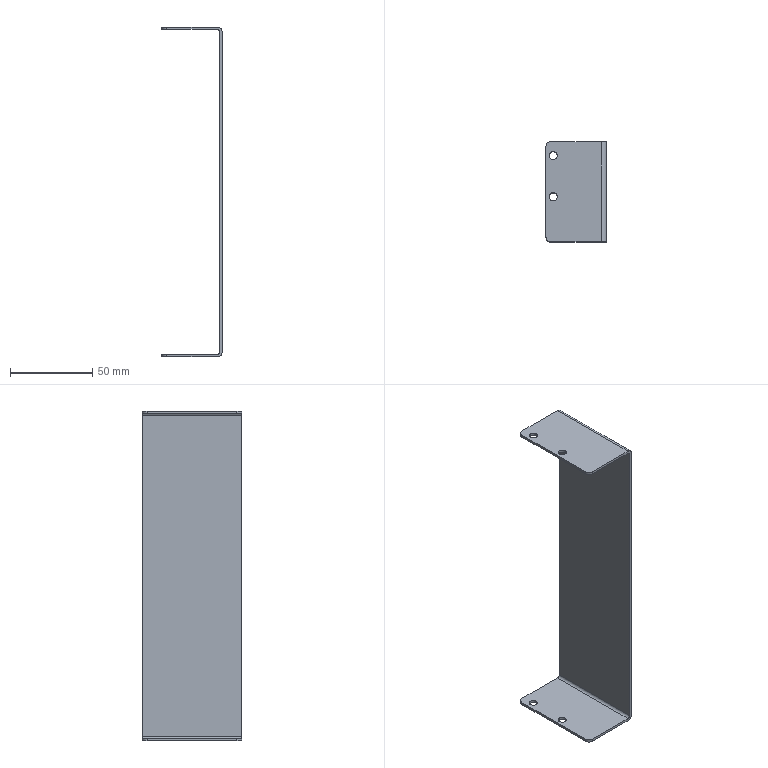Part | SolidWorks | features BaseBody 1 | 1 solid | 26 faces | box 36.5 x 60.5 x 200 mm | volume 24198 mm3 | cylinder 16 | plane 10 | commonest cylinder face diameters 5 x8 6 x6 3 x2
STEP:
#1=CARTESIAN_POINT('',(310.979,1928.044,-20.5));
#2=VERTEX_POINT('',#1);
#3=CARTESIAN_POINT('',(305.979,1928.044,-20.5));
#4=VERTEX_POINT('',#3);
#5=CARTESIAN_POINT('',(308.479,1928.044,-20.5));
#6=DIRECTION('',(0.,0.,-1.));
#7=DIRECTION('',(-1.,0.,0.));
#8=AXIS2_PLACEMENT_3D('',#5,#6,#7);
#9=CIRCLE('',#8,2.5);
#10=EDGE_CURVE('',#2,#4,#9,.T.);
#11=ORIENTED_EDGE('',*,*,#10,.F.);
#12=CARTESIAN_POINT('',(310.979,1928.044,-22.));
#13=VERTEX_POINT('',#12);
#14=CARTESIAN_POINT('',(310.979,1928.044,-8.386));
#15=DIRECTION('',(0.,0.,-1.));
#16=VECTOR('',#15,1000.);
#17=LINE('',#14,#16);
#18=EDGE_CURVE('',#2,#13,#17,.T.);
#19=ORIENTED_EDGE('',*,*,#18,.T.);
#20=CARTESIAN_POINT('',(305.979,1928.044,-22.));
#21=VERTEX_POINT('',#20);
#22=CARTESIAN_POINT('',(308.479,1928.044,-22.));
#23=DIRECTION('',(0.,0.,-1.));
#24=DIRECTION('',(-1.,0.,0.));
#25=AXIS2_PLACEMENT_3D('',#22,#23,#24);
#26=CIRCLE('',#25,2.5);
#27=EDGE_CURVE('',#13,#21,#26,.T.);
#28=ORIENTED_EDGE('',*,*,#27,.T.);
#29=CARTESIAN_POINT('',(305.979,1928.044,-8.386));
#30=DIRECTION('',(0.,0.,-1.));
#31=VECTOR('',#30,1000.);
#32=LINE('',#29,#31);
#33=EDGE_CURVE('',#4,#21,#32,.T.);
#34=ORIENTED_EDGE('',*,*,#33,.F.);
#35=EDGE_LOOP('',(#11,#19,#28,#34));
#36=FACE_OUTER_BOUND('',#35,.T.);
#37=CARTESIAN_POINT('',(308.479,1928.044,-8.386));
#38=DIRECTION('',(0.,0.,-1.));
#39=DIRECTION('',(-1.,0.,0.));
#40=AXIS2_PLACEMENT_3D('',#37,#38,#39);
#41=CYLINDRICAL_SURFACE('',#40,2.5);
#42=ADVANCED_FACE('',(#36),#41,.F.);
#43=CARTESIAN_POINT('',(310.979,1903.044,-20.5));
#44=VERTEX_POINT('',#43);
#45=CARTESIAN_POINT('',(305.979,1903.044,-20.5));
#46=VERTEX_POINT('',#45);
#47=CARTESIAN_POINT('',(308.479,1903.044,-20.5));
#48=DIRECTION('',(0.,0.,-1.));
#49=DIRECTION('',(-1.,0.,0.));
#50=AXIS2_PLACEMENT_3D('',#47,#48,#49);
#51=CIRCLE('',#50,2.5);
#52=EDGE_CURVE('',#44,#46,#51,.T.);
#53=ORIENTED_EDGE('',*,*,#52,.F.);
#54=CARTESIAN_POINT('',(310.979,1903.044,-22.));
#55=VERTEX_POINT('',#54);
#56=CARTESIAN_POINT('',(310.979,1903.044,-8.386));
#57=DIRECTION('',(0.,0.,-1.));
#58=VECTOR('',#57,1000.);
#59=LINE('',#56,#58);
#60=EDGE_CURVE('',#44,#55,#59,.T.);
#61=ORIENTED_EDGE('',*,*,#60,.T.);
#62=CARTESIAN_POINT('',(305.979,1903.044,-22.));
#63=VERTEX_POINT('',#62);
#64=CARTESIAN_POINT('',(308.479,1903.044,-22.));
#65=DIRECTION('',(0.,0.,-1.));
#66=DIRECTION('',(-1.,0.,0.));
#67=AXIS2_PLACEMENT_3D('',#64,#65,#66);
#68=CIRCLE('',#67,2.5);
#69=EDGE_CURVE('',#55,#63,#68,.T.);
#70=ORIENTED_EDGE('',*,*,#69,.T.);
#71=CARTESIAN_POINT('',(305.979,1903.044,-8.386));
#72=DIRECTION('',(0.,0.,-1.));
#73=VECTOR('',#72,1000.);
#74=LINE('',#71,#73);
#75=EDGE_CURVE('',#46,#63,#74,.T.);
#76=ORIENTED_EDGE('',*,*,#75,.F.);
#77=EDGE_LOOP('',(#53,#61,#70,#76));
#78=FACE_OUTER_BOUND('',#77,.T.);
#79=CARTESIAN_POINT('',(308.479,1903.044,-8.386));
#80=DIRECTION('',(0.,0.,-1.));
#81=DIRECTION('',(-1.,0.,0.));
#82=AXIS2_PLACEMENT_3D('',#79,#80,#81);
#83=CYLINDRICAL_SURFACE('',#82,2.5);
#84=ADVANCED_FACE('',(#78),#83,.F.);
#85=CARTESIAN_POINT('',(310.979,1928.044,-219.));
#86=VERTEX_POINT('',#85);
#87=CARTESIAN_POINT('',(305.979,1928.044,-219.));
#88=VERTEX_POINT('',#87);
#89=CARTESIAN_POINT('',(308.479,1928.044,-219.));
#90=DIRECTION('',(0.,0.,-1.));
#91=DIRECTION('',(-1.,0.,0.));
#92=AXIS2_PLACEMENT_3D('',#89,#90,#91);
#93=CIRCLE('',#92,2.5);
#94=EDGE_CURVE('',#86,#88,#93,.T.);
#95=ORIENTED_EDGE('',*,*,#94,.F.);
#96=CARTESIAN_POINT('',(310.979,1928.044,-220.5));
#97=VERTEX_POINT('',#96);
#98=CARTESIAN_POINT('',(310.979,1928.044,-8.386));
#99=DIRECTION('',(0.,0.,-1.));
#100=VECTOR('',#99,1000.);
#101=LINE('',#98,#100);
#102=EDGE_CURVE('',#86,#97,#101,.T.);
#103=ORIENTED_EDGE('',*,*,#102,.T.);
#104=CARTESIAN_POINT('',(305.979,1928.044,-220.5));
#105=VERTEX_POINT('',#104);
#106=CARTESIAN_POINT('',(308.479,1928.044,-220.5));
#107=DIRECTION('',(0.,0.,-1.));
#108=DIRECTION('',(-1.,0.,0.));
#109=AXIS2_PLACEMENT_3D('',#106,#107,#108);
#110=CIRCLE('',#109,2.5);
#111=EDGE_CURVE('',#97,#105,#110,.T.);
#112=ORIENTED_EDGE('',*,*,#111,.T.);
#113=CARTESIAN_POINT('',(305.979,1928.044,-8.386));
#114=DIRECTION('',(0.,0.,-1.));
#115=VECTOR('',#114,1000.);
#116=LINE('',#113,#115);
#117=EDGE_CURVE('',#88,#105,#116,.T.);
#118=ORIENTED_EDGE('',*,*,#117,.F.);
#119=EDGE_LOOP('',(#95,#103,#112,#118));
#120=FACE_OUTER_BOUND('',#119,.T.);
#121=CARTESIAN_POINT('',(308.479,1928.044,-8.386));
#122=DIRECTION('',(0.,0.,-1.));
#123=DIRECTION('',(-1.,0.,0.));
#124=AXIS2_PLACEMENT_3D('',#121,#122,#123);
#125=CYLINDRICAL_SURFACE('',#124,2.5);
#126=ADVANCED_FACE('',(#120),#125,.F.);
#127=CARTESIAN_POINT('',(310.979,1903.044,-219.));
#128=VERTEX_POINT('',#127);
#129=CARTESIAN_POINT('',(305.979,1903.044,-219.));
#130=VERTEX_POINT('',#129);
#131=CARTESIAN_POINT('',(308.479,1903.044,-219.));
#132=DIRECTION('',(0.,0.,-1.));
#133=DIRECTION('',(-1.,0.,0.));
#134=AXIS2_PLACEMENT_3D('',#131,#132,#133);
#135=CIRCLE('',#134,2.5);
#136=EDGE_CURVE('',#128,#130,#135,.T.);
#137=ORIENTED_EDGE('',*,*,#136,.F.);
#138=CARTESIAN_POINT('',(310.979,1903.044,-220.5));
#139=VERTEX_POINT('',#138);
#140=CARTESIAN_POINT('',(310.979,1903.044,-8.386));
#141=DIRECTION('',(0.,0.,-1.));
#142=VECTOR('',#141,1000.);
#143=LINE('',#140,#142);
#144=EDGE_CURVE('',#128,#139,#143,.T.);
#145=ORIENTED_EDGE('',*,*,#144,.T.);
#146=CARTESIAN_POINT('',(305.979,1903.044,-220.5));
#147=VERTEX_POINT('',#146);
#148=CARTESIAN_POINT('',(308.479,1903.044,-220.5));
#149=DIRECTION('',(0.,0.,-1.));
#150=DIRECTION('',(-1.,0.,0.));
#151=AXIS2_PLACEMENT_3D('',#148,#149,#150);
#152=CIRCLE('',#151,2.5);
#153=EDGE_CURVE('',#139,#147,#152,.T.);
#154=ORIENTED_EDGE('',*,*,#153,.T.);
#155=CARTESIAN_POINT('',(305.979,1903.044,-8.386));
#156=DIRECTION('',(0.,0.,-1.));
#157=VECTOR('',#156,1000.);
#158=LINE('',#155,#157);
#159=EDGE_CURVE('',#130,#147,#158,.T.);
#160=ORIENTED_EDGE('',*,*,#159,.F.);
#161=EDGE_LOOP('',(#137,#145,#154,#160));
#162=FACE_OUTER_BOUND('',#161,.T.);
#163=CARTESIAN_POINT('',(308.479,1903.044,-8.386));
#164=DIRECTION('',(0.,0.,-1.));
#165=DIRECTION('',(-1.,0.,0.));
#166=AXIS2_PLACEMENT_3D('',#163,#164,#165);
#167=CYLINDRICAL_SURFACE('',#166,2.5);
#168=ADVANCED_FACE('',(#162),#167,.F.);
#169=CARTESIAN_POINT('',(340.479,1936.294,-217.5));
#170=VERTEX_POINT('',#169);
#171=CARTESIAN_POINT('',(340.479,1936.294,-23.5));
#172=VERTEX_POINT('',#171);
#173=CARTESIAN_POINT('',(340.479,1936.294,-120.5));
#174=DIRECTION('',(0.,0.,1.));
#175=VECTOR('',#174,1000.);
#176=LINE('',#173,#175);
#177=EDGE_CURVE('',#170,#172,#176,.T.);
#178=ORIENTED_EDGE('',*,*,#177,.T.);
#179=CARTESIAN_POINT('',(340.479,1875.794,-23.5));
#180=VERTEX_POINT('',#179);
#181=CARTESIAN_POINT('',(340.479,1906.044,-23.5));
#182=DIRECTION('',(0.,-1.,0.));
#183=VECTOR('',#182,1000.);
#184=LINE('',#181,#183);
#185=EDGE_CURVE('',#172,#180,#184,.T.);
#186=ORIENTED_EDGE('',*,*,#185,.T.);
#187=CARTESIAN_POINT('',(340.479,1875.794,-217.5));
#188=VERTEX_POINT('',#187);
#189=CARTESIAN_POINT('',(340.479,1875.794,-120.5));
#190=DIRECTION('',(0.,0.,-1.));
#191=VECTOR('',#190,1000.);
#192=LINE('',#189,#191);
#193=EDGE_CURVE('',#180,#188,#192,.T.);
#194=ORIENTED_EDGE('',*,*,#193,.T.);
#195=CARTESIAN_POINT('',(340.479,1906.044,-217.5));
#196=DIRECTION('',(0.,1.,0.));
#197=VECTOR('',#196,1000.);
#198=LINE('',#195,#197);
#199=EDGE_CURVE('',#188,#170,#198,.T.);
#200=ORIENTED_EDGE('',*,*,#199,.T.);
#201=EDGE_LOOP('',(#178,#186,#194,#200));
#202=FACE_OUTER_BOUND('',#201,.T.);
#203=CARTESIAN_POINT('',(340.479,1906.044,-120.5));
#204=DIRECTION('',(1.,0.,0.));
#205=DIRECTION('',(0.,0.,-1.));
#206=AXIS2_PLACEMENT_3D('',#203,#204,#205);
#207=PLANE('',#206);
#208=ADVANCED_FACE('',(#202),#207,.T.);
#209=CARTESIAN_POINT('',(337.479,1875.794,-20.5));
#210=VERTEX_POINT('',#209);
#211=CARTESIAN_POINT('',(337.479,1875.794,-23.5));
#212=DIRECTION('',(0.,1.,0.));
#213=DIRECTION('',(0.,0.,-1.));
#214=AXIS2_PLACEMENT_3D('',#211,#212,#213);
#215=CIRCLE('',#214,3.);
#216=EDGE_CURVE('',#210,#180,#215,.T.);
#217=ORIENTED_EDGE('',*,*,#216,.T.);
#218=ORIENTED_EDGE('',*,*,#185,.F.);
#219=CARTESIAN_POINT('',(337.479,1936.294,-20.5));
#220=VERTEX_POINT('',#219);
#221=CARTESIAN_POINT('',(337.479,1936.294,-23.5));
#222=DIRECTION('',(0.,-1.,0.));
#223=DIRECTION('',(0.,0.,-1.));
#224=AXIS2_PLACEMENT_3D('',#221,#222,#223);
#225=CIRCLE('',#224,3.);
#226=EDGE_CURVE('',#172,#220,#225,.T.);
#227=ORIENTED_EDGE('',*,*,#226,.T.);
#228=CARTESIAN_POINT('',(337.479,1906.044,-20.5));
#229=DIRECTION('',(0.,-1.,0.));
#230=VECTOR('',#229,1000.);
#231=LINE('',#228,#230);
#232=EDGE_CURVE('',#220,#210,#231,.T.);
#233=ORIENTED_EDGE('',*,*,#232,.T.);
#234=EDGE_LOOP('',(#217,#218,#227,#233));
#235=FACE_OUTER_BOUND('',#234,.T.);
#236=CARTESIAN_POINT('',(337.479,1906.044,-23.5));
#237=DIRECTION('',(0.,-1.,0.));
#238=DIRECTION('',(0.,0.,-1.));
#239=AXIS2_PLACEMENT_3D('',#236,#237,#238);
#240=CYLINDRICAL_SURFACE('',#239,3.);
#241=ADVANCED_FACE('',(#235),#240,.T.);
#242=CARTESIAN_POINT('',(338.979,1936.294,-217.5));
#243=VERTEX_POINT('',#242);
#244=CARTESIAN_POINT('',(338.979,1936.294,-23.5));
#245=VERTEX_POINT('',#244);
#246=CARTESIAN_POINT('',(338.979,1936.294,-20.5));
#247=DIRECTION('',(0.,0.,1.));
#248=VECTOR('',#247,1000.);
#249=LINE('',#246,#248);
#250=EDGE_CURVE('',#243,#245,#249,.T.);
#251=ORIENTED_EDGE('',*,*,#250,.T.);
#252=CARTESIAN_POINT('',(337.479,1936.294,-22.));
#253=VERTEX_POINT('',#252);
#254=CARTESIAN_POINT('',(337.479,1936.294,-23.5));
#255=DIRECTION('',(0.,-1.,0.));
#256=DIRECTION('',(0.,0.,-1.));
#257=AXIS2_PLACEMENT_3D('',#254,#255,#256);
#258=CIRCLE('',#257,1.5);
#259=EDGE_CURVE('',#245,#253,#258,.T.);
#260=ORIENTED_EDGE('',*,*,#259,.T.);
#261=CARTESIAN_POINT('',(306.979,1936.294,-22.));
#262=VERTEX_POINT('',#261);
#263=CARTESIAN_POINT('',(338.979,1936.294,-22.));
#264=DIRECTION('',(-1.,0.,0.));
#265=VECTOR('',#264,1000.);
#266=LINE('',#263,#265);
#267=EDGE_CURVE('',#253,#262,#266,.T.);
#268=ORIENTED_EDGE('',*,*,#267,.T.);
#269=CARTESIAN_POINT('',(306.979,1936.294,-20.5));
#270=VERTEX_POINT('',#269);
#271=CARTESIAN_POINT('',(306.979,1936.294,-20.5));
#272=DIRECTION('',(0.,0.,1.));
#273=VECTOR('',#272,1000.);
#274=LINE('',#271,#273);
#275=EDGE_CURVE('',#262,#270,#274,.T.);
#276=ORIENTED_EDGE('',*,*,#275,.T.);
#277=CARTESIAN_POINT('',(338.979,1936.294,-20.5));
#278=DIRECTION('',(1.,0.,0.));
#279=VECTOR('',#278,1000.);
#280=LINE('',#277,#279);
#281=EDGE_CURVE('',#270,#220,#280,.T.);
#282=ORIENTED_EDGE('',*,*,#281,.T.);
#283=ORIENTED_EDGE('',*,*,#226,.F.);
#284=ORIENTED_EDGE('',*,*,#177,.F.);
#285=CARTESIAN_POINT('',(337.479,1936.294,-220.5));
#286=VERTEX_POINT('',#285);
#287=CARTESIAN_POINT('',(337.479,1936.294,-217.5));
#288=DIRECTION('',(0.,1.,0.));
#289=DIRECTION('',(0.,0.,1.));
#290=AXIS2_PLACEMENT_3D('',#287,#288,#289);
#291=CIRCLE('',#290,3.);
#292=EDGE_CURVE('',#170,#286,#291,.T.);
#293=ORIENTED_EDGE('',*,*,#292,.T.);
#294=CARTESIAN_POINT('',(306.979,1936.294,-220.5));
#295=VERTEX_POINT('',#294);
#296=CARTESIAN_POINT('',(338.979,1936.294,-220.5));
#297=DIRECTION('',(-1.,0.,0.));
#298=VECTOR('',#297,1000.);
#299=LINE('',#296,#298);
#300=EDGE_CURVE('',#286,#295,#299,.T.);
#301=ORIENTED_EDGE('',*,*,#300,.T.);
#302=CARTESIAN_POINT('',(306.979,1936.294,-219.));
#303=VERTEX_POINT('',#302);
#304=CARTESIAN_POINT('',(306.979,1936.294,-20.5));
#305=DIRECTION('',(0.,0.,1.));
#306=VECTOR('',#305,1000.);
#307=LINE('',#304,#306);
#308=EDGE_CURVE('',#295,#303,#307,.T.);
#309=ORIENTED_EDGE('',*,*,#308,.T.);
#310=CARTESIAN_POINT('',(337.479,1936.294,-219.));
#311=VERTEX_POINT('',#310);
#312=CARTESIAN_POINT('',(338.979,1936.294,-219.));
#313=DIRECTION('',(1.,0.,0.));
#314=VECTOR('',#313,1000.);
#315=LINE('',#312,#314);
#316=EDGE_CURVE('',#303,#311,#315,.T.);
#317=ORIENTED_EDGE('',*,*,#316,.T.);
#318=CARTESIAN_POINT('',(337.479,1936.294,-217.5));
#319=DIRECTION('',(0.,-1.,0.));
#320=DIRECTION('',(0.,0.,1.));
#321=AXIS2_PLACEMENT_3D('',#318,#319,#320);
#322=CIRCLE('',#321,1.5);
#323=EDGE_CURVE('',#311,#243,#322,.T.);
#324=ORIENTED_EDGE('',*,*,#323,.T.);
#325=EDGE_LOOP('',(#251,#260,#268,#276,#282,#283,#284,#293,#301,#309,#317,#324));
#326=FACE_OUTER_BOUND('',#325,.T.);
#327=CARTESIAN_POINT('',(338.979,1936.294,-20.5));
#328=DIRECTION('',(0.,1.,0.));
#329=DIRECTION('',(0.,0.,1.));
#330=AXIS2_PLACEMENT_3D('',#327,#328,#329);
#331=PLANE('',#330);
#332=ADVANCED_FACE('',(#326),#331,.T.);
#333=ORIENTED_EDGE('',*,*,#292,.F.);
#334=ORIENTED_EDGE('',*,*,#199,.F.);
#335=CARTESIAN_POINT('',(337.479,1875.794,-220.5));
#336=VERTEX_POINT('',#335);
#337=CARTESIAN_POINT('',(337.479,1875.794,-217.5));
#338=DIRECTION('',(0.,1.,0.));
#339=DIRECTION('',(0.,0.,1.));
#340=AXIS2_PLACEMENT_3D('',#337,#338,#339);
#341=CIRCLE('',#340,3.);
#342=EDGE_CURVE('',#188,#336,#341,.T.);
#343=ORIENTED_EDGE('',*,*,#342,.T.);
#344=CARTESIAN_POINT('',(337.479,1906.044,-220.5));
#345=DIRECTION('',(0.,1.,0.));
#346=VECTOR('',#345,1000.);
#347=LINE('',#344,#346);
#348=EDGE_CURVE('',#336,#286,#347,.T.);
#349=ORIENTED_EDGE('',*,*,#348,.T.);
#350=EDGE_LOOP('',(#333,#334,#343,#349));
#351=FACE_OUTER_BOUND('',#350,.T.);
#352=CARTESIAN_POINT('',(337.479,1906.044,-217.5));
#353=DIRECTION('',(0.,1.,0.));
#354=DIRECTION('',(0.,0.,1.));
#355=AXIS2_PLACEMENT_3D('',#352,#353,#354);
#356=CYLINDRICAL_SURFACE('',#355,3.);
#357=ADVANCED_FACE('',(#351),#356,.T.);
#358=ORIENTED_EDGE('',*,*,#193,.F.);
#359=ORIENTED_EDGE('',*,*,#216,.F.);
#360=CARTESIAN_POINT('',(306.979,1875.794,-20.5));
#361=VERTEX_POINT('',#360);
#362=CARTESIAN_POINT('',(338.979,1875.794,-20.5));
#363=DIRECTION('',(-1.,0.,0.));
#364=VECTOR('',#363,1000.);
#365=LINE('',#362,#364);
#366=EDGE_CURVE('',#210,#361,#365,.T.);
#367=ORIENTED_EDGE('',*,*,#366,.T.);
#368=CARTESIAN_POINT('',(306.979,1875.794,-22.));
#369=VERTEX_POINT('',#368);
#370=CARTESIAN_POINT('',(306.979,1875.794,-220.5));
#371=DIRECTION('',(0.,0.,-1.));
#372=VECTOR('',#371,1000.);
#373=LINE('',#370,#372);
#374=EDGE_CURVE('',#361,#369,#373,.T.);
#375=ORIENTED_EDGE('',*,*,#374,.T.);
#376=CARTESIAN_POINT('',(337.479,1875.794,-22.));
#377=VERTEX_POINT('',#376);
#378=CARTESIAN_POINT('',(338.979,1875.794,-22.));
#379=DIRECTION('',(1.,0.,0.));
#380=VECTOR('',#379,1000.);
#381=LINE('',#378,#380);
#382=EDGE_CURVE('',#369,#377,#381,.T.);
#383=ORIENTED_EDGE('',*,*,#382,.T.);
#384=CARTESIAN_POINT('',(338.979,1875.794,-23.5));
#385=VERTEX_POINT('',#384);
#386=CARTESIAN_POINT('',(337.479,1875.794,-23.5));
#387=DIRECTION('',(0.,1.,0.));
#388=DIRECTION('',(0.,0.,-1.));
#389=AXIS2_PLACEMENT_3D('',#386,#387,#388);
#390=CIRCLE('',#389,1.5);
#391=EDGE_CURVE('',#377,#385,#390,.T.);
#392=ORIENTED_EDGE('',*,*,#391,.T.);
#393=CARTESIAN_POINT('',(338.979,1875.794,-217.5));
#394=VERTEX_POINT('',#393);
#395=CARTESIAN_POINT('',(338.979,1875.794,-220.5));
#396=DIRECTION('',(0.,0.,-1.));
#397=VECTOR('',#396,1000.);
#398=LINE('',#395,#397);
#399=EDGE_CURVE('',#385,#394,#398,.T.);
#400=ORIENTED_EDGE('',*,*,#399,.T.);
#401=CARTESIAN_POINT('',(337.479,1875.794,-219.));
#402=VERTEX_POINT('',#401);
#403=CARTESIAN_POINT('',(337.479,1875.794,-217.5));
#404=DIRECTION('',(0.,1.,0.));
#405=DIRECTION('',(0.,0.,1.));
#406=AXIS2_PLACEMENT_3D('',#403,#404,#405);
#407=CIRCLE('',#406,1.5);
#408=EDGE_CURVE('',#394,#402,#407,.T.);
#409=ORIENTED_EDGE('',*,*,#408,.T.);
#410=CARTESIAN_POINT('',(306.979,1875.794,-219.));
#411=VERTEX_POINT('',#410);
#412=CARTESIAN_POINT('',(338.979,1875.794,-219.));
#413=DIRECTION('',(-1.,0.,0.));
#414=VECTOR('',#413,1000.);
#415=LINE('',#412,#414);
#416=EDGE_CURVE('',#402,#411,#415,.T.);
#417=ORIENTED_EDGE('',*,*,#416,.T.);
#418=CARTESIAN_POINT('',(306.979,1875.794,-220.5));
#419=VERTEX_POINT('',#418);
#420=CARTESIAN_POINT('',(306.979,1875.794,-220.5));
#421=DIRECTION('',(0.,0.,-1.));
#422=VECTOR('',#421,1000.);
#423=LINE('',#420,#422);
#424=EDGE_CURVE('',#411,#419,#423,.T.);
#425=ORIENTED_EDGE('',*,*,#424,.T.);
#426=CARTESIAN_POINT('',(338.979,1875.794,-220.5));
#427=DIRECTION('',(1.,0.,0.));
#428=VECTOR('',#427,1000.);
#429=LINE('',#426,#428);
#430=EDGE_CURVE('',#419,#336,#429,.T.);
#431=ORIENTED_EDGE('',*,*,#430,.T.);
#432=ORIENTED_EDGE('',*,*,#342,.F.);
#433=EDGE_LOOP('',(#358,#359,#367,#375,#383,#392,#400,#409,#417,#425,#431,#432));
#434=FACE_OUTER_BOUND('',#433,.T.);
#435=CARTESIAN_POINT('',(338.979,1875.794,-220.5));
#436=DIRECTION('',(0.,-1.,0.));
#437=DIRECTION('',(0.,0.,-1.));
#438=AXIS2_PLACEMENT_3D('',#435,#436,#437);
#439=PLANE('',#438);
#440=ADVANCED_FACE('',(#434),#439,.T.);
#441=CARTESIAN_POINT('',(308.479,1928.044,-20.5));
#442=DIRECTION('',(0.,0.,-1.));
#443=DIRECTION('',(-1.,0.,0.));
#444=AXIS2_PLACEMENT_3D('',#441,#442,#443);
#445=CIRCLE('',#444,2.5);
#446=EDGE_CURVE('',#4,#2,#445,.T.);
#447=ORIENTED_EDGE('',*,*,#446,.T.);
#448=ORIENTED_EDGE('',*,*,#10,.T.);
#449=EDGE_LOOP('',(#447,#448));
#450=FACE_BOUND('',#449,.T.);
#451=CARTESIAN_POINT('',(308.479,1903.044,-20.5));
#452=DIRECTION('',(0.,0.,-1.));
#453=DIRECTION('',(-1.,0.,0.));
#454=AXIS2_PLACEMENT_3D('',#451,#452,#453);
#455=CIRCLE('',#454,2.5);
#456=EDGE_CURVE('',#46,#44,#455,.T.);
#457=ORIENTED_EDGE('',*,*,#456,.T.);
#458=ORIENTED_EDGE('',*,*,#52,.T.);
#459=EDGE_LOOP('',(#457,#458));
#460=FACE_BOUND('',#459,.T.);
#461=ORIENTED_EDGE('',*,*,#366,.F.);
#462=ORIENTED_EDGE('',*,*,#232,.F.);
#463=ORIENTED_EDGE('',*,*,#281,.F.);
#464=CARTESIAN_POINT('',(303.979,1933.294,-20.5));
#465=VERTEX_POINT('',#464);
#466=CARTESIAN_POINT('',(306.979,1933.294,-20.5));
#467=DIRECTION('',(0.,0.,1.));
#468=DIRECTION('',(-1.,0.,0.));
#469=AXIS2_PLACEMENT_3D('',#466,#467,#468);
#470=CIRCLE('',#469,3.);
#471=EDGE_CURVE('',#270,#465,#470,.T.);
#472=ORIENTED_EDGE('',*,*,#471,.T.);
#473=CARTESIAN_POINT('',(303.979,1878.794,-20.5));
#474=VERTEX_POINT('',#473);
#475=CARTESIAN_POINT('',(303.979,1906.044,-20.5));
#476=DIRECTION('',(0.,-1.,0.));
#477=VECTOR('',#476,1000.);
#478=LINE('',#475,#477);
#479=EDGE_CURVE('',#465,#474,#478,.T.);
#480=ORIENTED_EDGE('',*,*,#479,.T.);
#481=CARTESIAN_POINT('',(306.979,1878.794,-20.5));
#482=DIRECTION('',(0.,0.,1.));
#483=DIRECTION('',(-1.,0.,0.));
#484=AXIS2_PLACEMENT_3D('',#481,#482,#483);
#485=CIRCLE('',#484,3.);
#486=EDGE_CURVE('',#474,#361,#485,.T.);
#487=ORIENTED_EDGE('',*,*,#486,.T.);
#488=EDGE_LOOP('',(#461,#462,#463,#472,#480,#487));
#489=FACE_OUTER_BOUND('',#488,.T.);
#490=CARTESIAN_POINT('',(322.229,1906.044,-20.5));
#491=DIRECTION('',(0.,0.,1.));
#492=DIRECTION('',(1.,0.,0.));
#493=AXIS2_PLACEMENT_3D('',#490,#491,#492);
#494=PLANE('',#493);
#495=ADVANCED_FACE('',(#450,#460,#489),#494,.T.);
#496=ORIENTED_EDGE('',*,*,#391,.F.);
#497=CARTESIAN_POINT('',(337.479,1906.044,-22.));
#498=DIRECTION('',(0.,-1.,0.));
#499=VECTOR('',#498,1000.);
#500=LINE('',#497,#499);
#501=EDGE_CURVE('',#253,#377,#500,.T.);
#502=ORIENTED_EDGE('',*,*,#501,.F.);
#503=ORIENTED_EDGE('',*,*,#259,.F.);
#504=CARTESIAN_POINT('',(338.979,1906.044,-23.5));
#505=DIRECTION('',(0.,1.,0.));
#506=VECTOR('',#505,1000.);
#507=LINE('',#504,#506);
#508=EDGE_CURVE('',#385,#245,#507,.T.);
#509=ORIENTED_EDGE('',*,*,#508,.F.);
#510=EDGE_LOOP('',(#496,#502,#503,#509));
#511=FACE_OUTER_BOUND('',#510,.T.);
#512=CARTESIAN_POINT('',(337.479,1906.044,-23.5));
#513=DIRECTION('',(0.,-1.,0.));
#514=DIRECTION('',(0.,0.,-1.));
#515=AXIS2_PLACEMENT_3D('',#512,#513,#514);
#516=CYLINDRICAL_SURFACE('',#515,1.5);
#517=ADVANCED_FACE('',(#511),#516,.F.);
#518=ORIENTED_EDGE('',*,*,#250,.F.);
#519=CARTESIAN_POINT('',(338.979,1906.044,-217.5));
#520=DIRECTION('',(0.,1.,0.));
#521=VECTOR('',#520,1000.);
#522=LINE('',#519,#521);
#523=EDGE_CURVE('',#394,#243,#522,.T.);
#524=ORIENTED_EDGE('',*,*,#523,.F.);
#525=ORIENTED_EDGE('',*,*,#399,.F.);
#526=ORIENTED_EDGE('',*,*,#508,.T.);
#527=EDGE_LOOP('',(#518,#524,#525,#526));
#528=FACE_OUTER_BOUND('',#527,.T.);
#529=CARTESIAN_POINT('',(338.979,1906.044,-120.5));
#530=DIRECTION('',(1.,0.,0.));
#531=DIRECTION('',(0.,0.,-1.));
#532=AXIS2_PLACEMENT_3D('',#529,#530,#531);
#533=PLANE('',#532);
#534=ADVANCED_FACE('',(#528),#533,.F.);
#535=ORIENTED_EDGE('',*,*,#323,.F.);
#536=CARTESIAN_POINT('',(337.479,1906.044,-219.));
#537=DIRECTION('',(0.,1.,0.));
#538=VECTOR('',#537,1000.);
#539=LINE('',#536,#538);
#540=EDGE_CURVE('',#402,#311,#539,.T.);
#541=ORIENTED_EDGE('',*,*,#540,.F.);
#542=ORIENTED_EDGE('',*,*,#408,.F.);
#543=ORIENTED_EDGE('',*,*,#523,.T.);
#544=EDGE_LOOP('',(#535,#541,#542,#543));
#545=FACE_OUTER_BOUND('',#544,.T.);
#546=CARTESIAN_POINT('',(337.479,1906.044,-217.5));
#547=DIRECTION('',(0.,1.,0.));
#548=DIRECTION('',(0.,0.,1.));
#549=AXIS2_PLACEMENT_3D('',#546,#547,#548);
#550=CYLINDRICAL_SURFACE('',#549,1.5);
#551=ADVANCED_FACE('',(#545),#550,.F.);
#552=CARTESIAN_POINT('',(308.479,1928.044,-219.));
#553=DIRECTION('',(0.,0.,-1.));
#554=DIRECTION('',(-1.,0.,0.));
#555=AXIS2_PLACEMENT_3D('',#552,#553,#554);
#556=CIRCLE('',#555,2.5);
#557=EDGE_CURVE('',#88,#86,#556,.T.);
#558=ORIENTED_EDGE('',*,*,#557,.T.);
#559=ORIENTED_EDGE('',*,*,#94,.T.);
#560=EDGE_LOOP('',(#558,#559));
#561=FACE_BOUND('',#560,.T.);
#562=CARTESIAN_POINT('',(308.479,1903.044,-219.));
#563=DIRECTION('',(0.,0.,-1.));
#564=DIRECTION('',(-1.,0.,0.));
#565=AXIS2_PLACEMENT_3D('',#562,#563,#564);
#566=CIRCLE('',#565,2.5);
#567=EDGE_CURVE('',#130,#128,#566,.T.);
#568=ORIENTED_EDGE('',*,*,#567,.T.);
#569=ORIENTED_EDGE('',*,*,#136,.T.);
#570=EDGE_LOOP('',(#568,#569));
#571=FACE_BOUND('',#570,.T.);
#572=ORIENTED_EDGE('',*,*,#316,.F.);
#573=CARTESIAN_POINT('',(303.979,1933.294,-219.));
#574=VERTEX_POINT('',#573);
#575=CARTESIAN_POINT('',(306.979,1933.294,-219.));
#576=DIRECTION('',(0.,0.,1.));
#577=DIRECTION('',(1.,0.,0.));
#578=AXIS2_PLACEMENT_3D('',#575,#576,#577);
#579=CIRCLE('',#578,3.);
#580=EDGE_CURVE('',#303,#574,#579,.T.);
#581=ORIENTED_EDGE('',*,*,#580,.T.);
#582=CARTESIAN_POINT('',(303.979,1878.794,-219.));
#583=VERTEX_POINT('',#582);
#584=CARTESIAN_POINT('',(303.979,1906.044,-219.));
#585=DIRECTION('',(0.,-1.,0.));
#586=VECTOR('',#585,1000.);
#587=LINE('',#584,#586);
#588=EDGE_CURVE('',#574,#583,#587,.T.);
#589=ORIENTED_EDGE('',*,*,#588,.T.);
#590=CARTESIAN_POINT('',(306.979,1878.794,-219.));
#591=DIRECTION('',(0.,0.,1.));
#592=DIRECTION('',(1.,0.,0.));
#593=AXIS2_PLACEMENT_3D('',#590,#591,#592);
#594=CIRCLE('',#593,3.);
#595=EDGE_CURVE('',#583,#411,#594,.T.);
#596=ORIENTED_EDGE('',*,*,#595,.T.);
#597=ORIENTED_EDGE('',*,*,#416,.F.);
#598=ORIENTED_EDGE('',*,*,#540,.T.);
#599=EDGE_LOOP('',(#572,#581,#589,#596,#597,#598));
#600=FACE_OUTER_BOUND('',#599,.T.);
#601=CARTESIAN_POINT('',(322.229,1906.044,-219.));
#602=DIRECTION('',(0.,0.,1.));
#603=DIRECTION('',(1.,0.,0.));
#604=AXIS2_PLACEMENT_3D('',#601,#602,#603);
#605=PLANE('',#604);
#606=ADVANCED_FACE('',(#561,#571,#600),#605,.T.);
#607=CARTESIAN_POINT('',(303.979,1933.294,-220.5));
#608=VERTEX_POINT('',#607);
#609=CARTESIAN_POINT('',(303.979,1933.294,-120.5));
#610=DIRECTION('',(0.,0.,1.));
#611=VECTOR('',#610,1000.);
#612=LINE('',#609,#611);
#613=EDGE_CURVE('',#608,#574,#612,.T.);
#614=ORIENTED_EDGE('',*,*,#613,.T.);
#615=ORIENTED_EDGE('',*,*,#580,.F.);
#616=ORIENTED_EDGE('',*,*,#308,.F.);
#617=CARTESIAN_POINT('',(306.979,1933.294,-220.5));
#618=DIRECTION('',(0.,0.,1.));
#619=DIRECTION('',(1.,0.,0.));
#620=AXIS2_PLACEMENT_3D('',#617,#618,#619);
#621=CIRCLE('',#620,3.);
#622=EDGE_CURVE('',#295,#608,#621,.T.);
#623=ORIENTED_EDGE('',*,*,#622,.T.);
#624=EDGE_LOOP('',(#614,#615,#616,#623));
#625=FACE_OUTER_BOUND('',#624,.T.);
#626=CARTESIAN_POINT('',(306.979,1933.294,-120.5));
#627=DIRECTION('',(0.,0.,1.));
#628=DIRECTION('',(1.,0.,0.));
#629=AXIS2_PLACEMENT_3D('',#626,#627,#628);
#630=CYLINDRICAL_SURFACE('',#629,3.);
#631=ADVANCED_FACE('',(#625),#630,.T.);
#632=CARTESIAN_POINT('',(308.479,1928.044,-220.5));
#633=DIRECTION('',(0.,0.,-1.));
#634=DIRECTION('',(-1.,0.,0.));
#635=AXIS2_PLACEMENT_3D('',#632,#633,#634);
#636=CIRCLE('',#635,2.5);
#637=EDGE_CURVE('',#105,#97,#636,.T.);
#638=ORIENTED_EDGE('',*,*,#637,.F.);
#639=ORIENTED_EDGE('',*,*,#111,.F.);
#640=EDGE_LOOP('',(#638,#639));
#641=FACE_BOUND('',#640,.T.);
#642=CARTESIAN_POINT('',(308.479,1903.044,-220.5));
#643=DIRECTION('',(0.,0.,-1.));
#644=DIRECTION('',(-1.,0.,0.));
#645=AXIS2_PLACEMENT_3D('',#642,#643,#644);
#646=CIRCLE('',#645,2.5);
#647=EDGE_CURVE('',#147,#139,#646,.T.);
#648=ORIENTED_EDGE('',*,*,#647,.F.);
#649=ORIENTED_EDGE('',*,*,#153,.F.);
#650=EDGE_LOOP('',(#648,#649));
#651=FACE_BOUND('',#650,.T.);
#652=ORIENTED_EDGE('',*,*,#300,.F.);
#653=ORIENTED_EDGE('',*,*,#348,.F.);
#654=ORIENTED_EDGE('',*,*,#430,.F.);
#655=CARTESIAN_POINT('',(303.979,1878.794,-220.5));
#656=VERTEX_POINT('',#655);
#657=CARTESIAN_POINT('',(306.979,1878.794,-220.5));
#658=DIRECTION('',(0.,0.,1.));
#659=DIRECTION('',(1.,0.,0.));
#660=AXIS2_PLACEMENT_3D('',#657,#658,#659);
#661=CIRCLE('',#660,3.);
#662=EDGE_CURVE('',#656,#419,#661,.T.);
#663=ORIENTED_EDGE('',*,*,#662,.F.);
#664=CARTESIAN_POINT('',(303.979,1906.044,-220.5));
#665=DIRECTION('',(0.,-1.,0.));
#666=VECTOR('',#665,1000.);
#667=LINE('',#664,#666);
#668=EDGE_CURVE('',#608,#656,#667,.T.);
#669=ORIENTED_EDGE('',*,*,#668,.F.);
#670=ORIENTED_EDGE('',*,*,#622,.F.);
#671=EDGE_LOOP('',(#652,#653,#654,#663,#669,#670));
#672=FACE_OUTER_BOUND('',#671,.T.);
#673=CARTESIAN_POINT('',(322.229,1906.044,-220.5));
#674=DIRECTION('',(0.,0.,1.));
#675=DIRECTION('',(1.,0.,0.));
#676=AXIS2_PLACEMENT_3D('',#673,#674,#675);
#677=PLANE('',#676);
#678=ADVANCED_FACE('',(#641,#651,#672),#677,.F.);
#679=ORIENTED_EDGE('',*,*,#275,.F.);
#680=CARTESIAN_POINT('',(303.979,1933.294,-22.));
#681=VERTEX_POINT('',#680);
#682=CARTESIAN_POINT('',(306.979,1933.294,-22.));
#683=DIRECTION('',(0.,0.,1.));
#684=DIRECTION('',(-1.,0.,0.));
#685=AXIS2_PLACEMENT_3D('',#682,#683,#684);
#686=CIRCLE('',#685,3.);
#687=EDGE_CURVE('',#262,#681,#686,.T.);
#688=ORIENTED_EDGE('',*,*,#687,.T.);
#689=CARTESIAN_POINT('',(303.979,1933.294,-20.5));
#690=DIRECTION('',(0.,0.,1.));
#691=VECTOR('',#690,1000.);
#692=LINE('',#689,#691);
#693=EDGE_CURVE('',#681,#465,#692,.T.);
#694=ORIENTED_EDGE('',*,*,#693,.T.);
#695=ORIENTED_EDGE('',*,*,#471,.F.);
#696=EDGE_LOOP('',(#679,#688,#694,#695));
#697=FACE_OUTER_BOUND('',#696,.T.);
#698=CARTESIAN_POINT('',(306.979,1933.294,-20.5));
#699=DIRECTION('',(0.,0.,-1.));
#700=DIRECTION('',(-1.,0.,0.));
#701=AXIS2_PLACEMENT_3D('',#698,#699,#700);
#702=CYLINDRICAL_SURFACE('',#701,3.);
#703=ADVANCED_FACE('',(#697),#702,.T.);
#704=CARTESIAN_POINT('',(308.479,1928.044,-22.));
#705=DIRECTION('',(0.,0.,-1.));
#706=DIRECTION('',(-1.,0.,0.));
#707=AXIS2_PLACEMENT_3D('',#704,#705,#706);
#708=CIRCLE('',#707,2.5);
#709=EDGE_CURVE('',#21,#13,#708,.T.);
#710=ORIENTED_EDGE('',*,*,#709,.F.);
#711=ORIENTED_EDGE('',*,*,#27,.F.);
#712=EDGE_LOOP('',(#710,#711));
#713=FACE_BOUND('',#712,.T.);
#714=CARTESIAN_POINT('',(308.479,1903.044,-22.));
#715=DIRECTION('',(0.,0.,-1.));
#716=DIRECTION('',(-1.,0.,0.));
#717=AXIS2_PLACEMENT_3D('',#714,#715,#716);
#718=CIRCLE('',#717,2.5);
#719=EDGE_CURVE('',#63,#55,#718,.T.);
#720=ORIENTED_EDGE('',*,*,#719,.F.);
#721=ORIENTED_EDGE('',*,*,#69,.F.);
#722=EDGE_LOOP('',(#720,#721));
#723=FACE_BOUND('',#722,.T.);
#724=ORIENTED_EDGE('',*,*,#382,.F.);
#725=CARTESIAN_POINT('',(303.979,1878.794,-22.));
#726=VERTEX_POINT('',#725);
#727=CARTESIAN_POINT('',(306.979,1878.794,-22.));
#728=DIRECTION('',(0.,0.,1.));
#729=DIRECTION('',(-1.,0.,0.));
#730=AXIS2_PLACEMENT_3D('',#727,#728,#729);
#731=CIRCLE('',#730,3.);
#732=EDGE_CURVE('',#726,#369,#731,.T.);
#733=ORIENTED_EDGE('',*,*,#732,.F.);
#734=CARTESIAN_POINT('',(303.979,1906.044,-22.));
#735=DIRECTION('',(0.,-1.,0.));
#736=VECTOR('',#735,1000.);
#737=LINE('',#734,#736);
#738=EDGE_CURVE('',#681,#726,#737,.T.);
#739=ORIENTED_EDGE('',*,*,#738,.F.);
#740=ORIENTED_EDGE('',*,*,#687,.F.);
#741=ORIENTED_EDGE('',*,*,#267,.F.);
#742=ORIENTED_EDGE('',*,*,#501,.T.);
#743=EDGE_LOOP('',(#724,#733,#739,#740,#741,#742));
#744=FACE_OUTER_BOUND('',#743,.T.);
#745=CARTESIAN_POINT('',(322.229,1906.044,-22.));
#746=DIRECTION('',(0.,0.,1.));
#747=DIRECTION('',(1.,0.,0.));
#748=AXIS2_PLACEMENT_3D('',#745,#746,#747);
#749=PLANE('',#748);
#750=ADVANCED_FACE('',(#713,#723,#744),#749,.F.);
#751=ORIENTED_EDGE('',*,*,#424,.F.);
#752=ORIENTED_EDGE('',*,*,#595,.F.);
#753=CARTESIAN_POINT('',(303.979,1878.794,-220.5));
#754=DIRECTION('',(0.,0.,-1.));
#755=VECTOR('',#754,1000.);
#756=LINE('',#753,#755);
#757=EDGE_CURVE('',#583,#656,#756,.T.);
#758=ORIENTED_EDGE('',*,*,#757,.T.);
#759=ORIENTED_EDGE('',*,*,#662,.T.);
#760=EDGE_LOOP('',(#751,#752,#758,#759));
#761=FACE_OUTER_BOUND('',#760,.T.);
#762=CARTESIAN_POINT('',(306.979,1878.794,-220.5));
#763=DIRECTION('',(0.,0.,1.));
#764=DIRECTION('',(1.,0.,0.));
#765=AXIS2_PLACEMENT_3D('',#762,#763,#764);
#766=CYLINDRICAL_SURFACE('',#765,3.);
#767=ADVANCED_FACE('',(#761),#766,.T.);
#768=CARTESIAN_POINT('',(303.979,1878.794,-120.5));
#769=DIRECTION('',(0.,0.,-1.));
#770=VECTOR('',#769,1000.);
#771=LINE('',#768,#770);
#772=EDGE_CURVE('',#474,#726,#771,.T.);
#773=ORIENTED_EDGE('',*,*,#772,.T.);
#774=ORIENTED_EDGE('',*,*,#732,.T.);
#775=ORIENTED_EDGE('',*,*,#374,.F.);
#776=ORIENTED_EDGE('',*,*,#486,.F.);
#777=EDGE_LOOP('',(#773,#774,#775,#776));
#778=FACE_OUTER_BOUND('',#777,.T.);
#779=CARTESIAN_POINT('',(306.979,1878.794,-120.5));
#780=DIRECTION('',(0.,0.,-1.));
#781=DIRECTION('',(-1.,0.,0.));
#782=AXIS2_PLACEMENT_3D('',#779,#780,#781);
#783=CYLINDRICAL_SURFACE('',#782,3.);
#784=ADVANCED_FACE('',(#778),#783,.T.);
#785=ORIENTED_EDGE('',*,*,#18,.F.);
#786=ORIENTED_EDGE('',*,*,#446,.F.);
#787=ORIENTED_EDGE('',*,*,#33,.T.);
#788=ORIENTED_EDGE('',*,*,#709,.T.);
#789=EDGE_LOOP('',(#785,#786,#787,#788));
#790=FACE_OUTER_BOUND('',#789,.T.);
#791=CARTESIAN_POINT('',(308.479,1928.044,-8.386));
#792=DIRECTION('',(0.,0.,-1.));
#793=DIRECTION('',(-1.,0.,0.));
#794=AXIS2_PLACEMENT_3D('',#791,#792,#793);
#795=CYLINDRICAL_SURFACE('',#794,2.5);
#796=ADVANCED_FACE('',(#790),#795,.F.);
#797=ORIENTED_EDGE('',*,*,#60,.F.);
#798=ORIENTED_EDGE('',*,*,#456,.F.);
#799=ORIENTED_EDGE('',*,*,#75,.T.);
#800=ORIENTED_EDGE('',*,*,#719,.T.);
#801=EDGE_LOOP('',(#797,#798,#799,#800));
#802=FACE_OUTER_BOUND('',#801,.T.);
#803=CARTESIAN_POINT('',(308.479,1903.044,-8.386));
#804=DIRECTION('',(0.,0.,-1.));
#805=DIRECTION('',(-1.,0.,0.));
#806=AXIS2_PLACEMENT_3D('',#803,#804,#805);
#807=CYLINDRICAL_SURFACE('',#806,2.5);
#808=ADVANCED_FACE('',(#802),#807,.F.);
#809=ORIENTED_EDGE('',*,*,#738,.T.);
#810=ORIENTED_EDGE('',*,*,#772,.F.);
#811=ORIENTED_EDGE('',*,*,#479,.F.);
#812=ORIENTED_EDGE('',*,*,#693,.F.);
#813=EDGE_LOOP('',(#809,#810,#811,#812));
#814=FACE_OUTER_BOUND('',#813,.T.);
#815=CARTESIAN_POINT('',(303.979,1936.294,-20.5));
#816=DIRECTION('',(-1.,0.,0.));
#817=DIRECTION('',(0.,0.,1.));
#818=AXIS2_PLACEMENT_3D('',#815,#816,#817);
#819=PLANE('',#818);
#820=ADVANCED_FACE('',(#814),#819,.T.);
#821=ORIENTED_EDGE('',*,*,#102,.F.);
#822=ORIENTED_EDGE('',*,*,#557,.F.);
#823=ORIENTED_EDGE('',*,*,#117,.T.);
#824=ORIENTED_EDGE('',*,*,#637,.T.);
#825=EDGE_LOOP('',(#821,#822,#823,#824));
#826=FACE_OUTER_BOUND('',#825,.T.);
#827=CARTESIAN_POINT('',(308.479,1928.044,-8.386));
#828=DIRECTION('',(0.,0.,-1.));
#829=DIRECTION('',(-1.,0.,0.));
#830=AXIS2_PLACEMENT_3D('',#827,#828,#829);
#831=CYLINDRICAL_SURFACE('',#830,2.5);
#832=ADVANCED_FACE('',(#826),#831,.F.);
#833=ORIENTED_EDGE('',*,*,#144,.F.);
#834=ORIENTED_EDGE('',*,*,#567,.F.);
#835=ORIENTED_EDGE('',*,*,#159,.T.);
#836=ORIENTED_EDGE('',*,*,#647,.T.);
#837=EDGE_LOOP('',(#833,#834,#835,#836));
#838=FACE_OUTER_BOUND('',#837,.T.);
#839=CARTESIAN_POINT('',(308.479,1903.044,-8.386));
#840=DIRECTION('',(0.,0.,-1.));
#841=DIRECTION('',(-1.,0.,0.));
#842=AXIS2_PLACEMENT_3D('',#839,#840,#841);
#843=CYLINDRICAL_SURFACE('',#842,2.5);
#844=ADVANCED_FACE('',(#838),#843,.F.);
#845=ORIENTED_EDGE('',*,*,#588,.F.);
#846=ORIENTED_EDGE('',*,*,#613,.F.);
#847=ORIENTED_EDGE('',*,*,#668,.T.);
#848=ORIENTED_EDGE('',*,*,#757,.F.);
#849=EDGE_LOOP('',(#845,#846,#847,#848));
#850=FACE_OUTER_BOUND('',#849,.T.);
#851=CARTESIAN_POINT('',(303.979,1875.794,-220.5));
#852=DIRECTION('',(-1.,0.,0.));
#853=DIRECTION('',(0.,0.,1.));
#854=AXIS2_PLACEMENT_3D('',#851,#852,#853);
#855=PLANE('',#854);
#856=ADVANCED_FACE('',(#850),#855,.T.);
#857=CLOSED_SHELL('',(#42,#84,#126,#168,#208,#241,#332,#357,#440,#495,#517,#534,#551,#606,#631,#678,#703,#750,#767,#784,#796,#808,#820,#832,#844,#856));
#858=MANIFOLD_SOLID_BREP('',#857);
#859=CARTESIAN_POINT('',(0.,0.,0.));
#860=DIRECTION('',(0.,0.,1.));
#861=DIRECTION('',(1.,0.,0.));
#862=AXIS2_PLACEMENT_3D('',#859,#860,#861);
#863=(LENGTH_UNIT()NAMED_UNIT(*)SI_UNIT(.MILLI.,.METRE.));
#864=UNCERTAINTY_MEASURE_WITH_UNIT(LENGTH_MEASURE(0.00001),#863,'','');
#865=(NAMED_UNIT(*)PLANE_ANGLE_UNIT()SI_UNIT($,.RADIAN.));
#866=(NAMED_UNIT(*)SI_UNIT($,.STERADIAN.)SOLID_ANGLE_UNIT());
#867=(GEOMETRIC_REPRESENTATION_CONTEXT(3)GLOBAL_UNCERTAINTY_ASSIGNED_CONTEXT((#864))GLOBAL_UNIT_ASSIGNED_CONTEXT((#863,#865,#866))REPRESENTATION_CONTEXT('',''));
#868=ADVANCED_BREP_SHAPE_REPRESENTATION('',(#858,#862),#867);